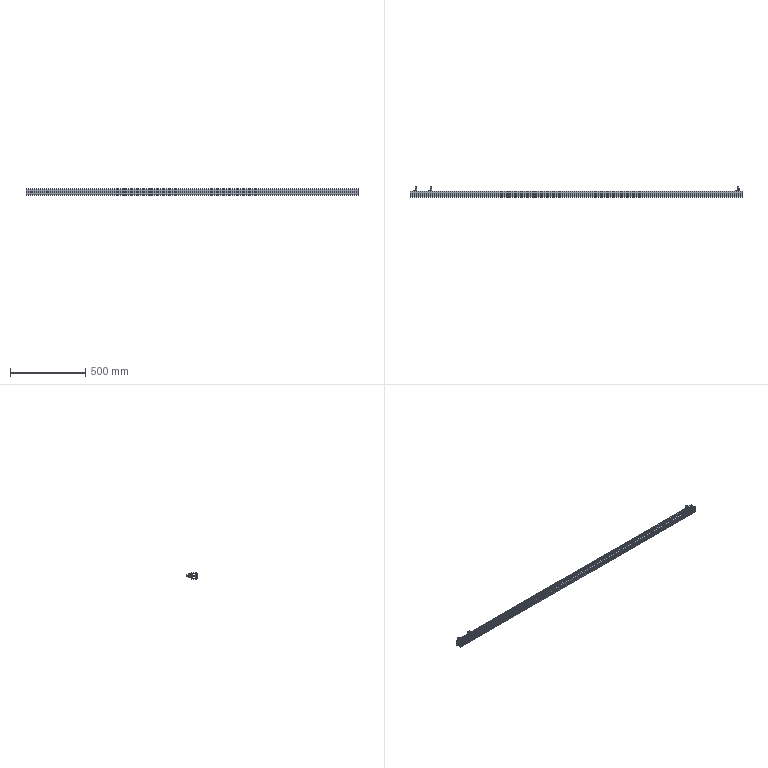Part | SolidWorks | features LocalLPattern 1, ReferencePattern 1 | 7 solids | 383 faces | box 2200 x 69.8 x 40 mm | volume 1056150 mm3 | plane 295 | cylinder 88 | commonest cylinder face diameters 3.2 x24 2.5 x18 3.8 x12 4 x12 6.5 x6 5 x4